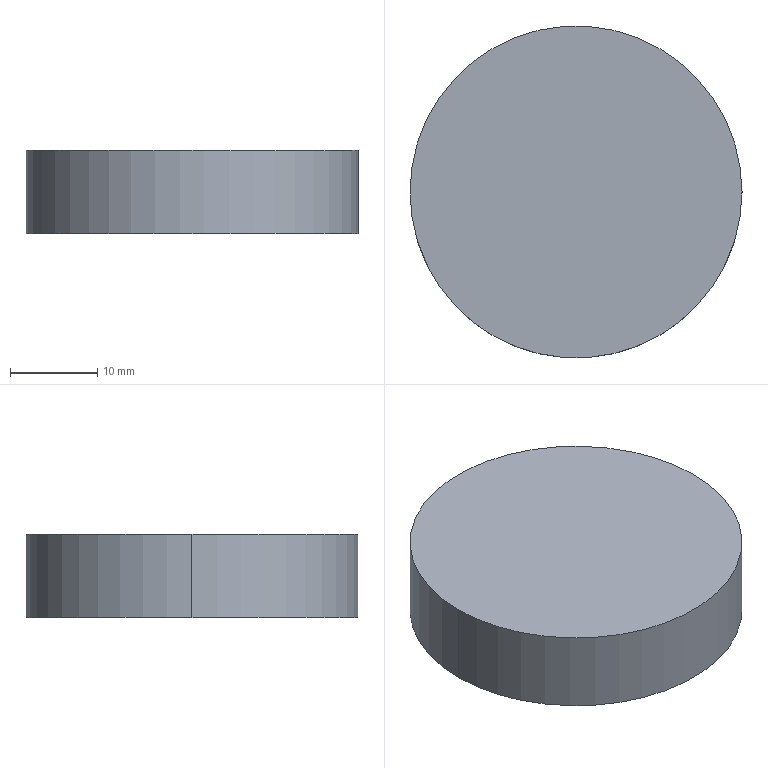Part | SolidWorks | features Extrusion 1 | 1 solid | 4 faces | box 38.1 x 38.1 x 9.525 mm | volume 10859 mm3 | cylinder 2 | plane 2 | commonest cylinder face diameters 38.1 x2
STEP:
#1=CARTESIAN_POINT('',(19.05,0.,9.525));
#2=VERTEX_POINT('',#1);
#3=CARTESIAN_POINT('',(-19.05,0.,9.525));
#4=VERTEX_POINT('',#3);
#5=CARTESIAN_POINT('',(0.,0.,9.525));
#6=DIRECTION('',(0.,0.,1.));
#7=DIRECTION('',(1.,0.,0.));
#8=AXIS2_PLACEMENT_3D('',#5,#6,#7);
#9=CIRCLE('',#8,19.05);
#10=EDGE_CURVE('',#2,#4,#9,.T.);
#11=ORIENTED_EDGE('',*,*,#10,.F.);
#12=CARTESIAN_POINT('',(19.05,0.,0.));
#13=VERTEX_POINT('',#12);
#14=CARTESIAN_POINT('',(19.05,0.,9.525));
#15=DIRECTION('',(0.,0.,-1.));
#16=VECTOR('',#15,1000.);
#17=LINE('',#14,#16);
#18=EDGE_CURVE('',#2,#13,#17,.T.);
#19=ORIENTED_EDGE('',*,*,#18,.T.);
#20=CARTESIAN_POINT('',(-19.05,0.,0.));
#21=VERTEX_POINT('',#20);
#22=CARTESIAN_POINT('',(0.,0.,0.));
#23=DIRECTION('',(0.,0.,1.));
#24=DIRECTION('',(1.,0.,0.));
#25=AXIS2_PLACEMENT_3D('',#22,#23,#24);
#26=CIRCLE('',#25,19.05);
#27=EDGE_CURVE('',#13,#21,#26,.T.);
#28=ORIENTED_EDGE('',*,*,#27,.T.);
#29=CARTESIAN_POINT('',(-19.05,0.,9.525));
#30=DIRECTION('',(0.,0.,-1.));
#31=VECTOR('',#30,1000.);
#32=LINE('',#29,#31);
#33=EDGE_CURVE('',#4,#21,#32,.T.);
#34=ORIENTED_EDGE('',*,*,#33,.F.);
#35=EDGE_LOOP('',(#11,#19,#28,#34));
#36=FACE_OUTER_BOUND('',#35,.T.);
#37=CARTESIAN_POINT('',(0.,0.,9.525));
#38=DIRECTION('',(0.,0.,-1.));
#39=DIRECTION('',(-1.,0.,0.));
#40=AXIS2_PLACEMENT_3D('',#37,#38,#39);
#41=CYLINDRICAL_SURFACE('',#40,19.05);
#42=ADVANCED_FACE('',(#36),#41,.T.);
#43=ORIENTED_EDGE('',*,*,#18,.F.);
#44=CARTESIAN_POINT('',(0.,0.,9.525));
#45=DIRECTION('',(0.,0.,1.));
#46=DIRECTION('',(1.,0.,0.));
#47=AXIS2_PLACEMENT_3D('',#44,#45,#46);
#48=CIRCLE('',#47,19.05);
#49=EDGE_CURVE('',#4,#2,#48,.T.);
#50=ORIENTED_EDGE('',*,*,#49,.F.);
#51=ORIENTED_EDGE('',*,*,#33,.T.);
#52=CARTESIAN_POINT('',(0.,0.,0.));
#53=DIRECTION('',(0.,0.,1.));
#54=DIRECTION('',(1.,0.,0.));
#55=AXIS2_PLACEMENT_3D('',#52,#53,#54);
#56=CIRCLE('',#55,19.05);
#57=EDGE_CURVE('',#21,#13,#56,.T.);
#58=ORIENTED_EDGE('',*,*,#57,.T.);
#59=EDGE_LOOP('',(#43,#50,#51,#58));
#60=FACE_OUTER_BOUND('',#59,.T.);
#61=CARTESIAN_POINT('',(0.,0.,9.525));
#62=DIRECTION('',(0.,0.,-1.));
#63=DIRECTION('',(-1.,0.,0.));
#64=AXIS2_PLACEMENT_3D('',#61,#62,#63);
#65=CYLINDRICAL_SURFACE('',#64,19.05);
#66=ADVANCED_FACE('',(#60),#65,.T.);
#67=ORIENTED_EDGE('',*,*,#49,.T.);
#68=ORIENTED_EDGE('',*,*,#10,.T.);
#69=EDGE_LOOP('',(#67,#68));
#70=FACE_OUTER_BOUND('',#69,.T.);
#71=CARTESIAN_POINT('',(0.,0.,9.525));
#72=DIRECTION('',(0.,0.,1.));
#73=DIRECTION('',(1.,0.,0.));
#74=AXIS2_PLACEMENT_3D('',#71,#72,#73);
#75=PLANE('',#74);
#76=ADVANCED_FACE('',(#70),#75,.T.);
#77=ORIENTED_EDGE('',*,*,#57,.F.);
#78=ORIENTED_EDGE('',*,*,#27,.F.);
#79=EDGE_LOOP('',(#77,#78));
#80=FACE_OUTER_BOUND('',#79,.T.);
#81=CARTESIAN_POINT('',(0.,0.,0.));
#82=DIRECTION('',(0.,0.,1.));
#83=DIRECTION('',(1.,0.,0.));
#84=AXIS2_PLACEMENT_3D('',#81,#82,#83);
#85=PLANE('',#84);
#86=ADVANCED_FACE('',(#80),#85,.F.);
#87=CLOSED_SHELL('',(#42,#66,#76,#86));
#88=MANIFOLD_SOLID_BREP('',#87);
#89=CARTESIAN_POINT('',(0.,0.,0.));
#90=DIRECTION('',(0.,0.,1.));
#91=DIRECTION('',(1.,0.,0.));
#92=AXIS2_PLACEMENT_3D('',#89,#90,#91);
#93=(LENGTH_UNIT()NAMED_UNIT(*)SI_UNIT(.MILLI.,.METRE.));
#94=UNCERTAINTY_MEASURE_WITH_UNIT(LENGTH_MEASURE(0.00001),#93,'','');
#95=(NAMED_UNIT(*)PLANE_ANGLE_UNIT()SI_UNIT($,.RADIAN.));
#96=(NAMED_UNIT(*)SI_UNIT($,.STERADIAN.)SOLID_ANGLE_UNIT());
#97=(GEOMETRIC_REPRESENTATION_CONTEXT(3)GLOBAL_UNCERTAINTY_ASSIGNED_CONTEXT((#94))GLOBAL_UNIT_ASSIGNED_CONTEXT((#93,#95,#96))REPRESENTATION_CONTEXT('',''));
#98=ADVANCED_BREP_SHAPE_REPRESENTATION('',(#88,#92),#97);